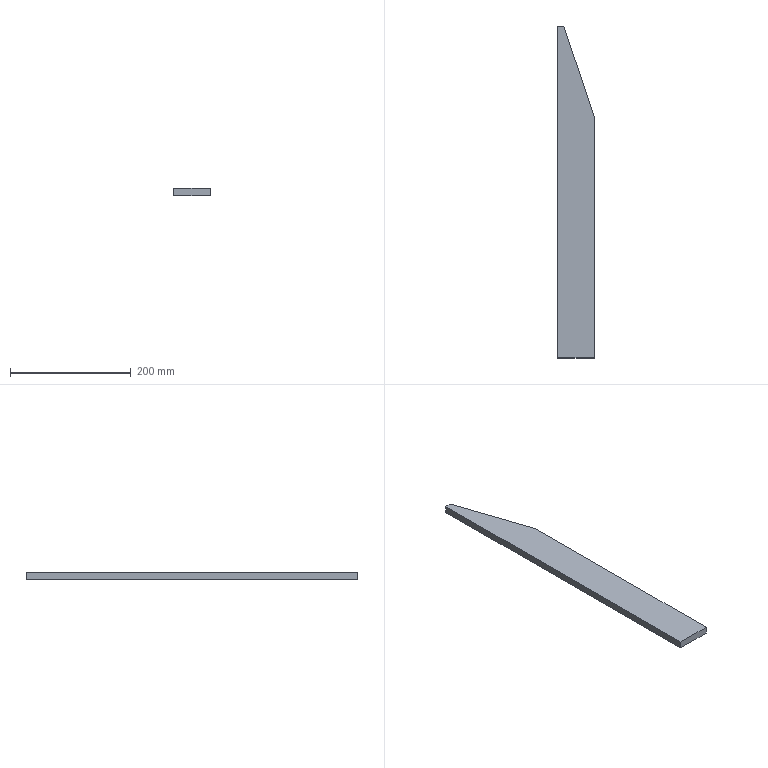Part | SolidWorks | features Extrusion 1, ICE 1 | 1 solid | 7 faces | box 60 x 550 x 12 mm | volume 351000 mm3 | plane 7
STEP:
#1=CARTESIAN_POINT('',(-30.,275.,0.));
#2=VERTEX_POINT('',#1);
#3=CARTESIAN_POINT('',(-30.,-275.,0.));
#4=VERTEX_POINT('',#3);
#5=CARTESIAN_POINT('',(-30.,275.,0.));
#6=DIRECTION('',(0.,-1.,0.));
#7=VECTOR('',#6,1000.);
#8=LINE('',#5,#7);
#9=EDGE_CURVE('',#2,#4,#8,.T.);
#10=ORIENTED_EDGE('',*,*,#9,.T.);
#11=CARTESIAN_POINT('',(-30.,-275.,12.));
#12=VERTEX_POINT('',#11);
#13=CARTESIAN_POINT('',(-30.,-275.,12.));
#14=DIRECTION('',(0.,0.,-1.));
#15=VECTOR('',#14,1000.);
#16=LINE('',#13,#15);
#17=EDGE_CURVE('',#12,#4,#16,.T.);
#18=ORIENTED_EDGE('',*,*,#17,.F.);
#19=CARTESIAN_POINT('',(-30.,275.,12.));
#20=VERTEX_POINT('',#19);
#21=CARTESIAN_POINT('',(-30.,275.,12.));
#22=DIRECTION('',(0.,-1.,0.));
#23=VECTOR('',#22,1000.);
#24=LINE('',#21,#23);
#25=EDGE_CURVE('',#20,#12,#24,.T.);
#26=ORIENTED_EDGE('',*,*,#25,.F.);
#27=CARTESIAN_POINT('',(-30.,275.,12.));
#28=DIRECTION('',(0.,0.,-1.));
#29=VECTOR('',#28,1000.);
#30=LINE('',#27,#29);
#31=EDGE_CURVE('',#20,#2,#30,.T.);
#32=ORIENTED_EDGE('',*,*,#31,.T.);
#33=EDGE_LOOP('',(#10,#18,#26,#32));
#34=FACE_OUTER_BOUND('',#33,.T.);
#35=CARTESIAN_POINT('',(-30.,275.,12.));
#36=DIRECTION('',(1.,0.,0.));
#37=DIRECTION('',(0.,1.,0.));
#38=AXIS2_PLACEMENT_3D('',#35,#36,#37);
#39=PLANE('',#38);
#40=ADVANCED_FACE('',(#34),#39,.F.);
#41=CARTESIAN_POINT('',(30.,-275.,0.));
#42=VERTEX_POINT('',#41);
#43=CARTESIAN_POINT('',(30.,-275.,0.));
#44=DIRECTION('',(1.,0.,0.));
#45=VECTOR('',#44,1000.);
#46=LINE('',#43,#45);
#47=EDGE_CURVE('',#4,#42,#46,.T.);
#48=ORIENTED_EDGE('',*,*,#47,.T.);
#49=CARTESIAN_POINT('',(30.,-275.,12.));
#50=VERTEX_POINT('',#49);
#51=CARTESIAN_POINT('',(30.,-275.,12.));
#52=DIRECTION('',(0.,0.,-1.));
#53=VECTOR('',#52,1000.);
#54=LINE('',#51,#53);
#55=EDGE_CURVE('',#50,#42,#54,.T.);
#56=ORIENTED_EDGE('',*,*,#55,.F.);
#57=CARTESIAN_POINT('',(30.,-275.,12.));
#58=DIRECTION('',(1.,0.,0.));
#59=VECTOR('',#58,1000.);
#60=LINE('',#57,#59);
#61=EDGE_CURVE('',#12,#50,#60,.T.);
#62=ORIENTED_EDGE('',*,*,#61,.F.);
#63=ORIENTED_EDGE('',*,*,#17,.T.);
#64=EDGE_LOOP('',(#48,#56,#62,#63));
#65=FACE_OUTER_BOUND('',#64,.T.);
#66=CARTESIAN_POINT('',(30.,-275.,12.));
#67=DIRECTION('',(0.,1.,0.));
#68=DIRECTION('',(0.,0.,1.));
#69=AXIS2_PLACEMENT_3D('',#66,#67,#68);
#70=PLANE('',#69);
#71=ADVANCED_FACE('',(#65),#70,.F.);
#72=CARTESIAN_POINT('',(30.,125.,0.));
#73=VERTEX_POINT('',#72);
#74=CARTESIAN_POINT('',(30.,275.,0.));
#75=DIRECTION('',(0.,1.,0.));
#76=VECTOR('',#75,1000.);
#77=LINE('',#74,#76);
#78=EDGE_CURVE('',#42,#73,#77,.T.);
#79=ORIENTED_EDGE('',*,*,#78,.T.);
#80=CARTESIAN_POINT('',(30.,125.,12.));
#81=VERTEX_POINT('',#80);
#82=CARTESIAN_POINT('',(30.,125.,0.));
#83=DIRECTION('',(0.,0.,1.));
#84=VECTOR('',#83,1000.);
#85=LINE('',#82,#84);
#86=EDGE_CURVE('',#73,#81,#85,.T.);
#87=ORIENTED_EDGE('',*,*,#86,.T.);
#88=CARTESIAN_POINT('',(30.,275.,12.));
#89=DIRECTION('',(0.,1.,0.));
#90=VECTOR('',#89,1000.);
#91=LINE('',#88,#90);
#92=EDGE_CURVE('',#50,#81,#91,.T.);
#93=ORIENTED_EDGE('',*,*,#92,.F.);
#94=ORIENTED_EDGE('',*,*,#55,.T.);
#95=EDGE_LOOP('',(#79,#87,#93,#94));
#96=FACE_OUTER_BOUND('',#95,.T.);
#97=CARTESIAN_POINT('',(30.,275.,12.));
#98=DIRECTION('',(-1.,0.,0.));
#99=DIRECTION('',(0.,-1.,0.));
#100=AXIS2_PLACEMENT_3D('',#97,#98,#99);
#101=PLANE('',#100);
#102=ADVANCED_FACE('',(#96),#101,.F.);
#103=CARTESIAN_POINT('',(-20.,275.,12.));
#104=VERTEX_POINT('',#103);
#105=CARTESIAN_POINT('',(30.,275.,12.));
#106=DIRECTION('',(-1.,0.,0.));
#107=VECTOR('',#106,1000.);
#108=LINE('',#105,#107);
#109=EDGE_CURVE('',#104,#20,#108,.T.);
#110=ORIENTED_EDGE('',*,*,#109,.F.);
#111=CARTESIAN_POINT('',(-20.,275.,0.));
#112=VERTEX_POINT('',#111);
#113=CARTESIAN_POINT('',(-20.,275.,0.));
#114=DIRECTION('',(0.,0.,1.));
#115=VECTOR('',#114,1000.);
#116=LINE('',#113,#115);
#117=EDGE_CURVE('',#112,#104,#116,.T.);
#118=ORIENTED_EDGE('',*,*,#117,.F.);
#119=CARTESIAN_POINT('',(30.,275.,0.));
#120=DIRECTION('',(-1.,0.,0.));
#121=VECTOR('',#120,1000.);
#122=LINE('',#119,#121);
#123=EDGE_CURVE('',#112,#2,#122,.T.);
#124=ORIENTED_EDGE('',*,*,#123,.T.);
#125=ORIENTED_EDGE('',*,*,#31,.F.);
#126=EDGE_LOOP('',(#110,#118,#124,#125));
#127=FACE_OUTER_BOUND('',#126,.T.);
#128=CARTESIAN_POINT('',(30.,275.,12.));
#129=DIRECTION('',(0.,-1.,0.));
#130=DIRECTION('',(0.,0.,-1.));
#131=AXIS2_PLACEMENT_3D('',#128,#129,#130);
#132=PLANE('',#131);
#133=ADVANCED_FACE('',(#127),#132,.F.);
#134=ORIENTED_EDGE('',*,*,#92,.T.);
#135=CARTESIAN_POINT('',(-20.,275.,12.));
#136=DIRECTION('',(0.3162,-0.9487,0.));
#137=VECTOR('',#136,1000.);
#138=LINE('',#135,#137);
#139=EDGE_CURVE('',#104,#81,#138,.T.);
#140=ORIENTED_EDGE('',*,*,#139,.F.);
#141=ORIENTED_EDGE('',*,*,#109,.T.);
#142=ORIENTED_EDGE('',*,*,#25,.T.);
#143=ORIENTED_EDGE('',*,*,#61,.T.);
#144=EDGE_LOOP('',(#134,#140,#141,#142,#143));
#145=FACE_OUTER_BOUND('',#144,.T.);
#146=CARTESIAN_POINT('',(0.,0.,12.));
#147=DIRECTION('',(0.,0.,-1.));
#148=DIRECTION('',(-1.,0.,0.));
#149=AXIS2_PLACEMENT_3D('',#146,#147,#148);
#150=PLANE('',#149);
#151=ADVANCED_FACE('',(#145),#150,.F.);
#152=CARTESIAN_POINT('',(-20.,275.,0.));
#153=DIRECTION('',(0.3162,-0.9487,0.));
#154=VECTOR('',#153,1000.);
#155=LINE('',#152,#154);
#156=EDGE_CURVE('',#112,#73,#155,.T.);
#157=ORIENTED_EDGE('',*,*,#156,.T.);
#158=ORIENTED_EDGE('',*,*,#78,.F.);
#159=ORIENTED_EDGE('',*,*,#47,.F.);
#160=ORIENTED_EDGE('',*,*,#9,.F.);
#161=ORIENTED_EDGE('',*,*,#123,.F.);
#162=EDGE_LOOP('',(#157,#158,#159,#160,#161));
#163=FACE_OUTER_BOUND('',#162,.T.);
#164=CARTESIAN_POINT('',(0.,0.,0.));
#165=DIRECTION('',(0.,0.,-1.));
#166=DIRECTION('',(-1.,0.,0.));
#167=AXIS2_PLACEMENT_3D('',#164,#165,#166);
#168=PLANE('',#167);
#169=ADVANCED_FACE('',(#163),#168,.T.);
#170=ORIENTED_EDGE('',*,*,#139,.T.);
#171=ORIENTED_EDGE('',*,*,#86,.F.);
#172=ORIENTED_EDGE('',*,*,#156,.F.);
#173=ORIENTED_EDGE('',*,*,#117,.T.);
#174=EDGE_LOOP('',(#170,#171,#172,#173));
#175=FACE_OUTER_BOUND('',#174,.T.);
#176=CARTESIAN_POINT('',(-20.,275.,0.));
#177=DIRECTION('',(-0.9487,-0.3162,0.));
#178=DIRECTION('',(0.3162,-0.9487,0.));
#179=AXIS2_PLACEMENT_3D('',#176,#177,#178);
#180=PLANE('',#179);
#181=ADVANCED_FACE('',(#175),#180,.F.);
#182=CLOSED_SHELL('',(#40,#71,#102,#133,#151,#169,#181));
#183=MANIFOLD_SOLID_BREP('',#182);
#184=CARTESIAN_POINT('',(0.,0.,0.));
#185=DIRECTION('',(0.,0.,1.));
#186=DIRECTION('',(1.,0.,0.));
#187=AXIS2_PLACEMENT_3D('',#184,#185,#186);
#188=(LENGTH_UNIT()NAMED_UNIT(*)SI_UNIT(.MILLI.,.METRE.));
#189=UNCERTAINTY_MEASURE_WITH_UNIT(LENGTH_MEASURE(0.00001),#188,'','');
#190=(NAMED_UNIT(*)PLANE_ANGLE_UNIT()SI_UNIT($,.RADIAN.));
#191=(NAMED_UNIT(*)SI_UNIT($,.STERADIAN.)SOLID_ANGLE_UNIT());
#192=(GEOMETRIC_REPRESENTATION_CONTEXT(3)GLOBAL_UNCERTAINTY_ASSIGNED_CONTEXT((#189))GLOBAL_UNIT_ASSIGNED_CONTEXT((#188,#190,#191))REPRESENTATION_CONTEXT('',''));
#193=ADVANCED_BREP_SHAPE_REPRESENTATION('',(#183,#187),#192);